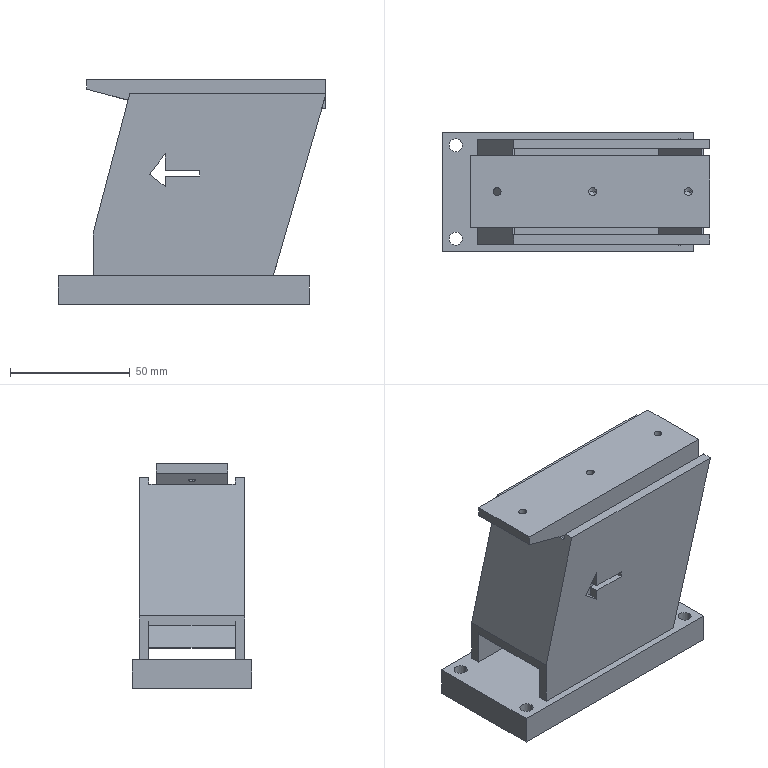Part | STEP file | 110 vibrator | 1 solid | 61 faces | box 112 x 50 x 94 mm | volume 146734 mm3 | plane 43 | cylinder 14 | cone 4 | commonest cylinder face diameters 5.5 x8 3.3 x6